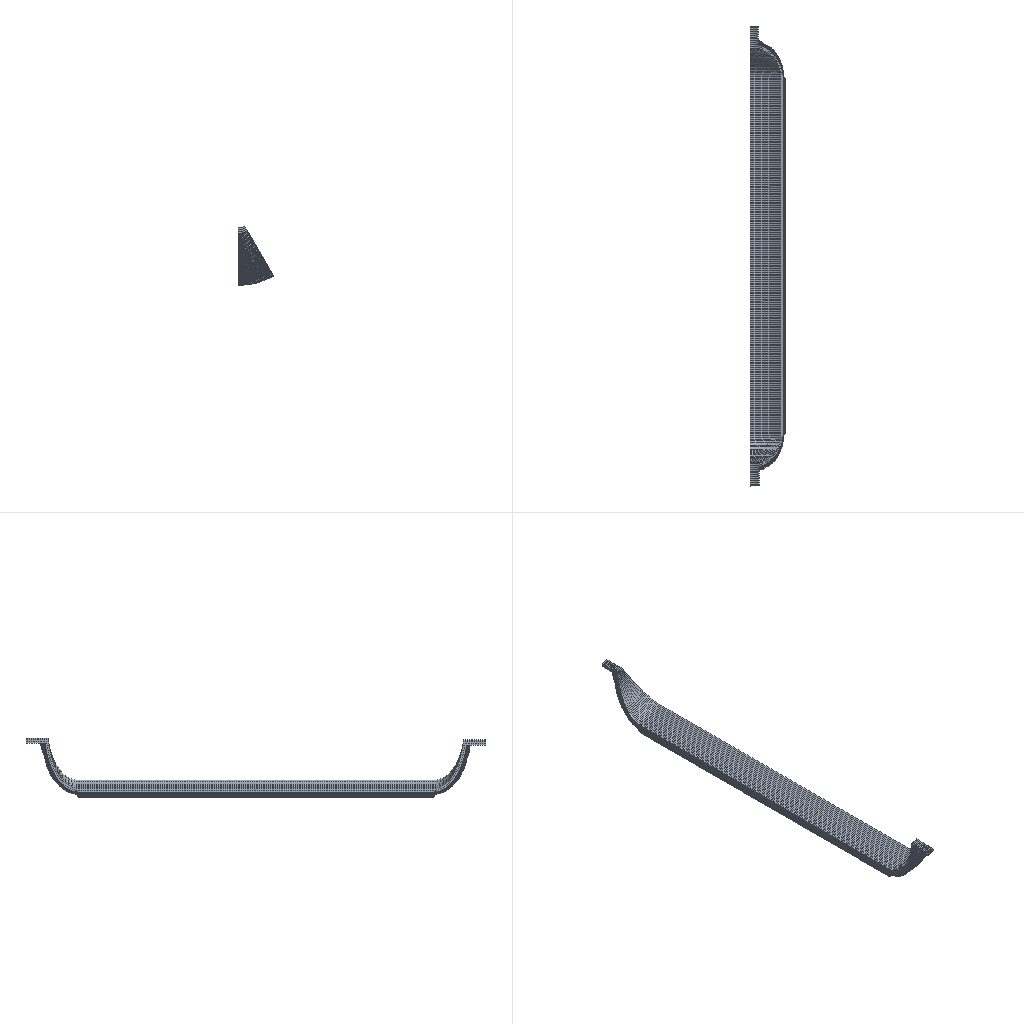Simulation study | abaqus
Set-up summary, first 205 of 324 lines:
category,name,step,type,value,unit,region
solver,abaqus
solver,version,,,Abaqus/Standard 3DEXPERIENCE R2017x
solver,version,,,Abaqus/Standard 3DEXPERIENCE R2017x
units,not stated in the deck,,not stated
analysis,deck1,,coupled temperature-displacement,coupled temperature-displacement
load_step,Step-1,Step-1,coupled temperature-displacement,nlgeom=True
contact,interactions,,,general=0 pairs=0 ties=1
load_step,requested,,,1
mesh,nodes,,,35039
mesh,elements,,,22287
element_type,C3D6T,,solid,1448
element_type,C3D8T,,solid,5175
element_type,C3D8RT,,solid,15664
load,load commands in deck,,count,2
bc,support commands in deck,,count,1
analysis,deck2,,static,static
load_step,Step-1,Step-1,static,nlgeom=True
contact,interactions,,,general=0 pairs=0 ties=1
load_step,requested,,,1
mesh,nodes,,,35039
mesh,elements,,,22287
element_type,C3D6,,solid,72
element_type,SC6R,,solid_shell,1376
element_type,SC8R,,solid_shell,15664
element_type,C3D8R,,solid,5175
load,load commands in deck,,count,2
bc,support commands in deck,,count,1
material,COMPOSITE,,in results
material,HDPE,,in results
material,T700,,in results
material,WCM_TANK1_MAT1_BIN0,,in results
material,WCM_TANK1_MAT1_BIN1,,in results
material,WCM_TANK1_MAT1_BIN10,,in results
material,WCM_TANK1_MAT1_BIN100,,in results
material,WCM_TANK1_MAT1_BIN101,,in results
material,WCM_TANK1_MAT1_BIN102,,in results
material,WCM_TANK1_MAT1_BIN103,,in results
material,WCM_TANK1_MAT1_BIN104,,in results
material,WCM_TANK1_MAT1_BIN105,,in results
material,WCM_TANK1_MAT1_BIN106,,in results
material,WCM_TANK1_MAT1_BIN107,,in results
material,WCM_TANK1_MAT1_BIN108,,in results
material,WCM_TANK1_MAT1_BIN109,,in results
material,WCM_TANK1_MAT1_BIN11,,in results
material,WCM_TANK1_MAT1_BIN110,,in results
material,WCM_TANK1_MAT1_BIN111,,in results
material,WCM_TANK1_MAT1_BIN112,,in results
material,WCM_TANK1_MAT1_BIN113,,in results
material,WCM_TANK1_MAT1_BIN114,,in results
material,WCM_TANK1_MAT1_BIN115,,in results
material,WCM_TANK1_MAT1_BIN116,,in results
material,WCM_TANK1_MAT1_BIN117,,in results
material,WCM_TANK1_MAT1_BIN119,,in results
material,WCM_TANK1_MAT1_BIN12,,in results
material,WCM_TANK1_MAT1_BIN120,,in results
material,WCM_TANK1_MAT1_BIN121,,in results
material,WCM_TANK1_MAT1_BIN123,,in results
material,WCM_TANK1_MAT1_BIN124,,in results
material,WCM_TANK1_MAT1_BIN125,,in results
material,WCM_TANK1_MAT1_BIN128,,in results
material,WCM_TANK1_MAT1_BIN129,,in results
material,WCM_TANK1_MAT1_BIN13,,in results
material,WCM_TANK1_MAT1_BIN130,,in results
material,WCM_TANK1_MAT1_BIN131,,in results
material,WCM_TANK1_MAT1_BIN132,,in results
material,WCM_TANK1_MAT1_BIN133,,in results
material,WCM_TANK1_MAT1_BIN134,,in results
material,WCM_TANK1_MAT1_BIN135,,in results
material,WCM_TANK1_MAT1_BIN136,,in results
material,WCM_TANK1_MAT1_BIN137,,in results
material,WCM_TANK1_MAT1_BIN14,,in results
material,WCM_TANK1_MAT1_BIN140,,in results
material,WCM_TANK1_MAT1_BIN142,,in results
material,WCM_TANK1_MAT1_BIN143,,in results
material,WCM_TANK1_MAT1_BIN144,,in results
material,WCM_TANK1_MAT1_BIN145,,in results
material,WCM_TANK1_MAT1_BIN15,,in results
material,WCM_TANK1_MAT1_BIN150,,in results
material,WCM_TANK1_MAT1_BIN151,,in results
material,WCM_TANK1_MAT1_BIN152,,in results
material,WCM_TANK1_MAT1_BIN156,,in results
material,WCM_TANK1_MAT1_BIN159,,in results
material,WCM_TANK1_MAT1_BIN16,,in results
material,WCM_TANK1_MAT1_BIN17,,in results
material,WCM_TANK1_MAT1_BIN18,,in results
material,WCM_TANK1_MAT1_BIN19,,in results
material,WCM_TANK1_MAT1_BIN2,,in results
material,WCM_TANK1_MAT1_BIN20,,in results
material,WCM_TANK1_MAT1_BIN21,,in results
material,WCM_TANK1_MAT1_BIN22,,in results
material,WCM_TANK1_MAT1_BIN23,,in results
material,WCM_TANK1_MAT1_BIN24,,in results
material,WCM_TANK1_MAT1_BIN25,,in results
material,WCM_TANK1_MAT1_BIN26,,in results
material,WCM_TANK1_MAT1_BIN27,,in results
material,WCM_TANK1_MAT1_BIN28,,in results
material,WCM_TANK1_MAT1_BIN29,,in results
material,WCM_TANK1_MAT1_BIN3,,in results
material,WCM_TANK1_MAT1_BIN30,,in results
material,WCM_TANK1_MAT1_BIN31,,in results
material,WCM_TANK1_MAT1_BIN32,,in results
material,WCM_TANK1_MAT1_BIN33,,in results
material,WCM_TANK1_MAT1_BIN34,,in results
material,WCM_TANK1_MAT1_BIN35,,in results
material,WCM_TANK1_MAT1_BIN36,,in results
material,WCM_TANK1_MAT1_BIN37,,in results
material,WCM_TANK1_MAT1_BIN38,,in results
material,WCM_TANK1_MAT1_BIN39,,in results
material,WCM_TANK1_MAT1_BIN4,,in results
material,WCM_TANK1_MAT1_BIN40,,in results
material,WCM_TANK1_MAT1_BIN41,,in results
material,WCM_TANK1_MAT1_BIN42,,in results
material,WCM_TANK1_MAT1_BIN43,,in results
material,WCM_TANK1_MAT1_BIN44,,in results
material,WCM_TANK1_MAT1_BIN45,,in results
material,WCM_TANK1_MAT1_BIN46,,in results
material,WCM_TANK1_MAT1_BIN47,,in results
material,WCM_TANK1_MAT1_BIN48,,in results
material,WCM_TANK1_MAT1_BIN49,,in results
material,WCM_TANK1_MAT1_BIN5,,in results
material,WCM_TANK1_MAT1_BIN50,,in results
material,WCM_TANK1_MAT1_BIN51,,in results
material,WCM_TANK1_MAT1_BIN52,,in results
material,WCM_TANK1_MAT1_BIN53,,in results
material,WCM_TANK1_MAT1_BIN54,,in results
material,WCM_TANK1_MAT1_BIN55,,in results
material,WCM_TANK1_MAT1_BIN56,,in results
material,WCM_TANK1_MAT1_BIN57,,in results
material,WCM_TANK1_MAT1_BIN58,,in results
material,WCM_TANK1_MAT1_BIN59,,in results
material,WCM_TANK1_MAT1_BIN6,,in results
material,WCM_TANK1_MAT1_BIN60,,in results
material,WCM_TANK1_MAT1_BIN61,,in results
material,WCM_TANK1_MAT1_BIN62,,in results
material,WCM_TANK1_MAT1_BIN63,,in results
material,WCM_TANK1_MAT1_BIN64,,in results
material,WCM_TANK1_MAT1_BIN65,,in results
material,WCM_TANK1_MAT1_BIN66,,in results
material,WCM_TANK1_MAT1_BIN67,,in results
material,WCM_TANK1_MAT1_BIN68,,in results
material,WCM_TANK1_MAT1_BIN69,,in results
material,WCM_TANK1_MAT1_BIN7,,in results
material,WCM_TANK1_MAT1_BIN70,,in results
material,WCM_TANK1_MAT1_BIN71,,in results
material,WCM_TANK1_MAT1_BIN72,,in results
material,WCM_TANK1_MAT1_BIN73,,in results
material,WCM_TANK1_MAT1_BIN74,,in results
material,WCM_TANK1_MAT1_BIN75,,in results
material,WCM_TANK1_MAT1_BIN76,,in results
material,WCM_TANK1_MAT1_BIN77,,in results
material,WCM_TANK1_MAT1_BIN78,,in results
material,WCM_TANK1_MAT1_BIN79,,in results
material,WCM_TANK1_MAT1_BIN8,,in results
material,WCM_TANK1_MAT1_BIN80,,in results
material,WCM_TANK1_MAT1_BIN81,,in results
material,WCM_TANK1_MAT1_BIN82,,in results
material,WCM_TANK1_MAT1_BIN83,,in results
material,WCM_TANK1_MAT1_BIN84,,in results
material,WCM_TANK1_MAT1_BIN85,,in results
material,WCM_TANK1_MAT1_BIN86,,in results
material,WCM_TANK1_MAT1_BIN87,,in results
material,WCM_TANK1_MAT1_BIN88,,in results
material,WCM_TANK1_MAT1_BIN89,,in results
material,WCM_TANK1_MAT1_BIN9,,in results
material,WCM_TANK1_MAT1_BIN90,,in results
material,WCM_TANK1_MAT1_BIN91,,in results
material,WCM_TANK1_MAT1_BIN92,,in results
material,WCM_TANK1_MAT1_BIN93,,in results
material,WCM_TANK1_MAT1_BIN94,,in results
material,WCM_TANK1_MAT1_BIN95,,in results
material,WCM_TANK1_MAT1_BIN96,,in results
material,WCM_TANK1_MAT1_BIN97,,in results
material,WCM_TANK1_MAT1_BIN98,,in results
material,WCM_TANK1_MAT1_BIN99,,in results
material,AAA,,in results
material,HDPE,,in results
material,T700,,in results
material,WCM_TANK1_MAT1_BIN0,,in results
material,WCM_TANK1_MAT1_BIN1,,in results
material,WCM_TANK1_MAT1_BIN10,,in results
material,WCM_TANK1_MAT1_BIN100,,in results
material,WCM_TANK1_MAT1_BIN101,,in results
material,WCM_TANK1_MAT1_BIN102,,in results
material,WCM_TANK1_MAT1_BIN103,,in results
material,WCM_TANK1_MAT1_BIN104,,in results
material,WCM_TANK1_MAT1_BIN105,,in results
material,WCM_TANK1_MAT1_BIN106,,in results
material,WCM_TANK1_MAT1_BIN107,,in results
material,WCM_TANK1_MAT1_BIN108,,in results
material,WCM_TANK1_MAT1_BIN109,,in results
material,WCM_TANK1_MAT1_BIN11,,in results
material,WCM_TANK1_MAT1_BIN110,,in results
material,WCM_TANK1_MAT1_BIN111,,in results
material,WCM_TANK1_MAT1_BIN112,,in results
material,WCM_TANK1_MAT1_BIN113,,in results
material,WCM_TANK1_MAT1_BIN114,,in results
material,WCM_TANK1_MAT1_BIN115,,in results
material,WCM_TANK1_MAT1_BIN116,,in results
material,WCM_TANK1_MAT1_BIN117,,in results
material,WCM_TANK1_MAT1_BIN119,,in results
material,WCM_TANK1_MAT1_BIN12,,in results
material,WCM_TANK1_MAT1_BIN120,,in results
material,WCM_TANK1_MAT1_BIN121,,in results
material,WCM_TANK1_MAT1_BIN123,,in results
Results summary:
result,step,,completed,increments=21 time=100.0/100.0
result,analysis,,,"coupled temperature-displacement, steady state"
result,last_loadstep,,,1
result,analysis steps,,count,1
result,primary field,,,"U, NT11"
result,reaction total,,FX,-2557.328,model units
result,reaction total,,FY,-21.753,model units
result,reaction total,,FZ,9533.795,model units
result,step,,completed,increments=21 time=10.0/10.0
result,analysis,,,static
result,last_loadstep,,,1
result,analysis steps,,count,1
result,primary field,,,U
result,reaction total,,FX,-2555.58,model units
result,reaction total,,FY,-23.777,model units
result,reaction total,,FZ,9537.58,model units